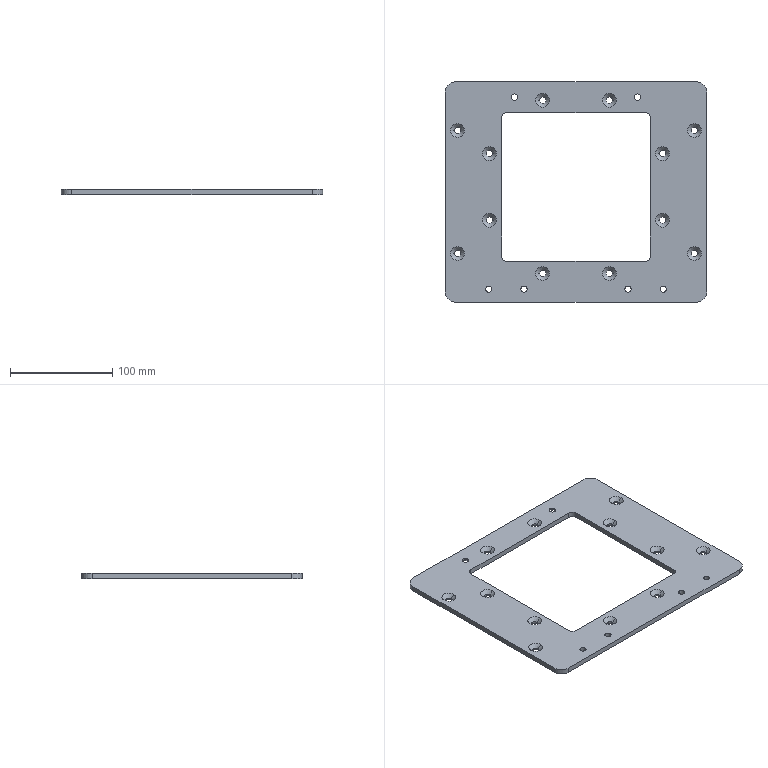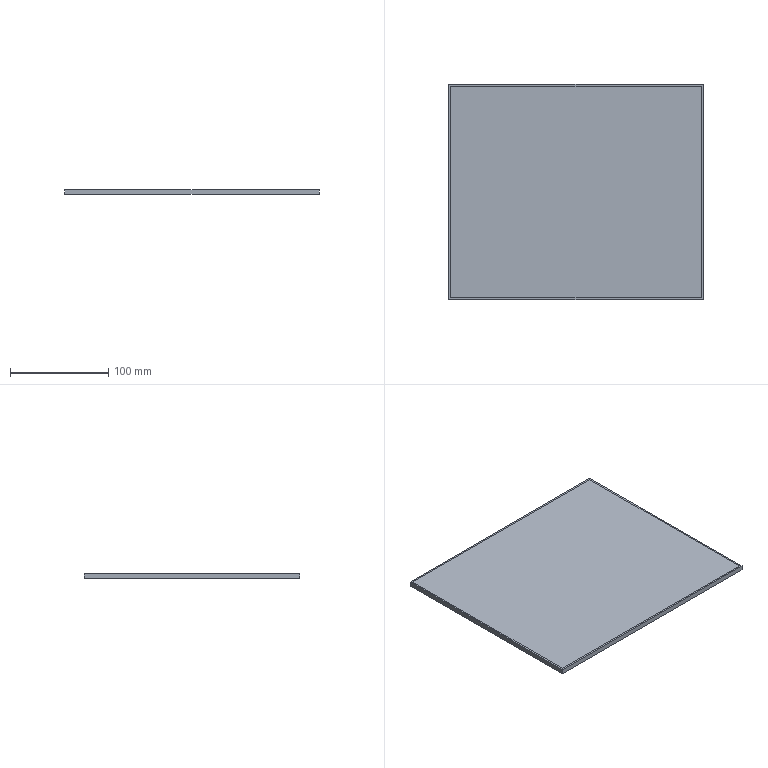CAM job | NX | 3-axis milling, drilling | part box 255 x 215 x 5 mm | stock box 259 x 219 x 5 mm
Tools:
number,name,description,diameter,corner_radius,flute_length,length,flutes
1,D6A45,Milling Tool-5 Parameters,6.0,0.0,50.0,75.0,2
10,6.5ZT,Drilling Tool,6.5,0.0,35.0,50.0,2
16,6.0ZT,Drilling Tool,6.0,0.0,35.0,50.0,2
15,D10,Milling Tool-5 Parameters,10.0,0.0,50.0,75.0,2
14,D10JING,Milling Tool-5 Parameters,10.0,0.0,50.0,75.0,2
Operations:
program,operation,operation_type,tool,method,geometry_group,spindle_rpm,surface_speed,feed_per_tooth,feed_cut,feed_plunge,cut_length_mm,path_length_mm,cut_time_min,machine_time_min
1,DRILLING,Operation,D6A45,METHOD,A,5000.0,94.0,0.035,350.0,0.0,72.0,1007.221,0.2057,0.2992
1,DRILLING_COPY,Operation,6.5ZT,METHOD,A,2000.0,40.0,0.075,300.0,0.0,160.339,1116.561,0.5345,0.6301
1,DRILLING_COPY_1,Operation,6.0ZT,METHOD,A,2000.0,37.0,0.0625,250.0,0.0,45.21,330.225,0.1808,0.2093
1,ZLEVEL_PROFILE_COPY_1,ZLevelMilling,D10,METHOD,A,9500.0,298.0,0.1053,2000.0,1000.0,4893.72,4955.52,2.467,2.473
1,ZLEVEL_PROFILE_COPY_1_COPY,ZLevelMilling,D10,METHOD,A,9500.0,298.0,0.1053,2000.0,1000.0,8634.455,8695.855,4.337,4.343
1,PLANAR_MILL_COPY_COPY_COPY_COPY,PlanarMilling,D6A45,METHOD,A,9500.0,179.0,0.0658,1250.0,100.0,1598.463,2683.22,1.279,1.387
1,ZLEVEL_PROFILE_COPY_1_COPY_1,ZLevelMilling,D6A45,METHOD,A,9500.0,179.0,0.0789,1500.0,1000.0,3118.963,4619.908,2.238,2.388
1,ZLEVEL_PROFILE_COPY_1_COPY_2,ZLevelMilling,D10JING,METHOD,A,9500.0,298.0,0.0789,1500.0,1000.0,2220.589,2282.389,1.5,1.506
1,ZLEVEL_PROFILE_COPY_1_COPY_COPY,ZLevelMilling,D10JING,METHOD,A,9500.0,298.0,0.0632,1200.0,1000.0,4778.698,4846.123,3.983,3.99
2,PLANAR_MILL_COPY_COPY_COPY_COPY_COPY,PlanarMilling,D6A45,METHOD,B,9500.0,179.0,0.0658,1250.0,100.0,1765.646,3663.428,1.413,1.602
2,ZLEVEL_PROFILE_COPY_1_COPY_1_COPY,ZLevelMilling,D6A45,METHOD,B,9500.0,179.0,0.0789,1500.0,1000.0,526.898,769.917,0.3777,0.402